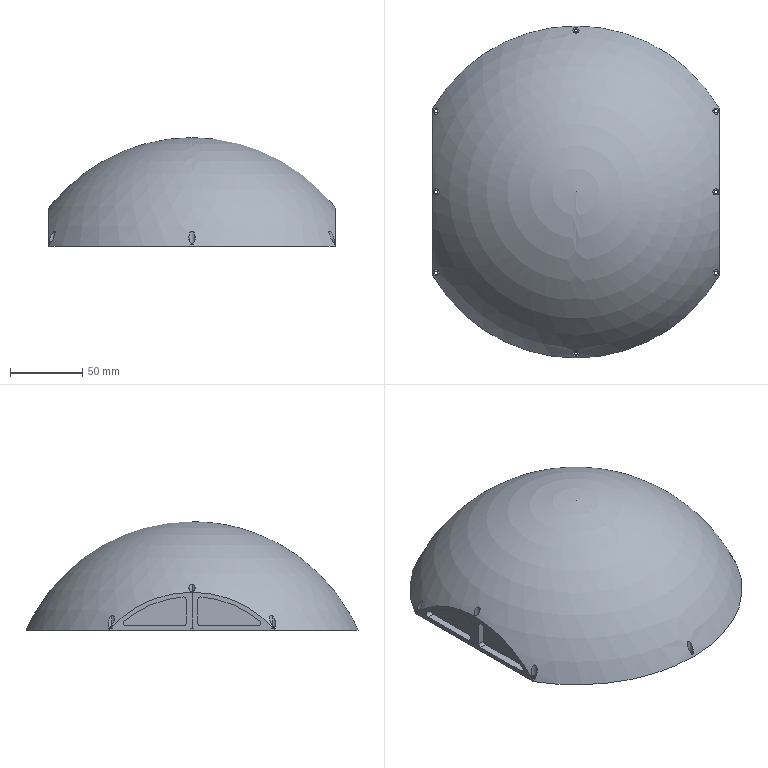Part | SolidWorks | features ICE 5, Cut 1, Fillet 1, MirrorPattern 1, Revolution 1, Shell 1 | 1 solid | 79 faces | box 198 x 229.129 x 75 mm | volume 135832 mm3 | cylinder 52 | plane 25 | sphere 2 | commonest cylinder face diameters 2.3 x16 4.2 x16 4 x14 146.63 x4 214.758 x2